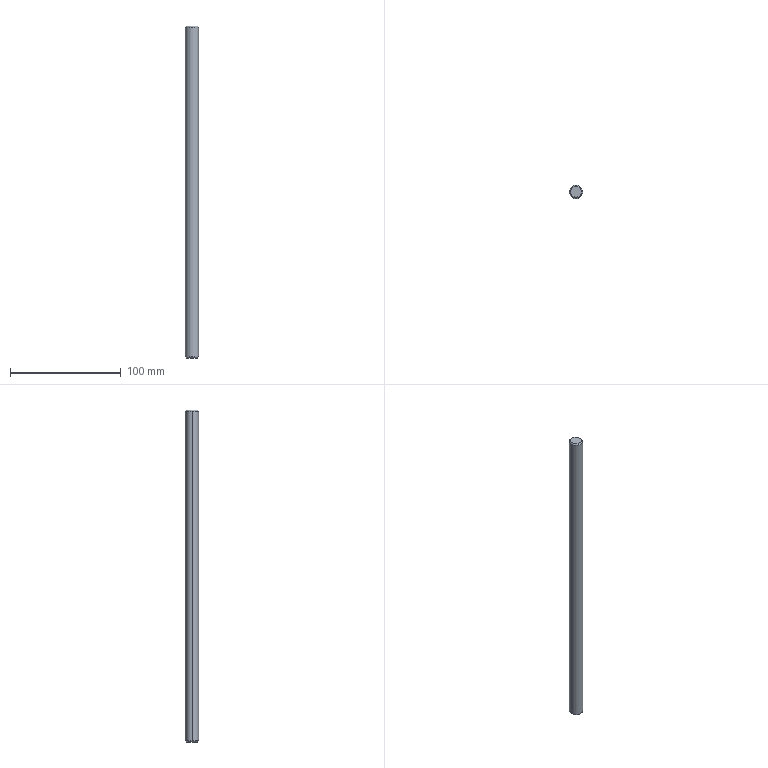Part | STEP file | X77b-01009 | 1 solid | 8 faces | box 12 x 12 x 300 mm | volume 33894 mm3 | cone 4 | cylinder 2 | plane 2 | commonest cylinder face diameters 12 x2
STEP:
#1=CARTESIAN_POINT('',(5.,2660.092,300.));
#2=VERTEX_POINT('',#1);
#3=CARTESIAN_POINT('',(-5.,2660.092,300.));
#4=VERTEX_POINT('',#3);
#5=CARTESIAN_POINT('',(0.000000001,2660.092,300.));
#6=DIRECTION('',(0.,0.,1.));
#7=DIRECTION('',(1.,0.,0.));
#8=AXIS2_PLACEMENT_3D('',#5,#6,#7);
#9=CIRCLE('',#8,5.);
#10=EDGE_CURVE('',#2,#4,#9,.T.);
#11=ORIENTED_EDGE('',*,*,#10,.F.);
#12=CARTESIAN_POINT('',(6.,2660.092,299.));
#13=VERTEX_POINT('',#12);
#14=CARTESIAN_POINT('',(5.,2660.092,300.));
#15=DIRECTION('',(0.7071,0.,-0.7071));
#16=VECTOR('',#15,1000.);
#17=LINE('',#14,#16);
#18=EDGE_CURVE('',#2,#13,#17,.T.);
#19=ORIENTED_EDGE('',*,*,#18,.T.);
#20=CARTESIAN_POINT('',(-6.,2660.092,299.));
#21=VERTEX_POINT('',#20);
#22=CARTESIAN_POINT('',(0.000000001,2660.092,299.));
#23=DIRECTION('',(0.,0.,-1.));
#24=DIRECTION('',(1.,0.,0.));
#25=AXIS2_PLACEMENT_3D('',#22,#23,#24);
#26=CIRCLE('',#25,6.);
#27=EDGE_CURVE('',#21,#13,#26,.T.);
#28=ORIENTED_EDGE('',*,*,#27,.F.);
#29=CARTESIAN_POINT('',(-5.,2660.092,300.));
#30=DIRECTION('',(-0.7071,0.,-0.7071));
#31=VECTOR('',#30,1000.);
#32=LINE('',#29,#31);
#33=EDGE_CURVE('',#4,#21,#32,.T.);
#34=ORIENTED_EDGE('',*,*,#33,.F.);
#35=EDGE_LOOP('',(#11,#19,#28,#34));
#36=FACE_OUTER_BOUND('',#35,.T.);
#37=CARTESIAN_POINT('',(0.000000001,2660.092,300.));
#38=DIRECTION('',(0.,0.,-1.));
#39=DIRECTION('',(-1.,0.,0.));
#40=AXIS2_PLACEMENT_3D('',#37,#38,#39);
#41=CONICAL_SURFACE('',#40,5.,0.7854);
#42=ADVANCED_FACE('',(#36),#41,.T.);
#43=CARTESIAN_POINT('',(-5.,2660.092,0.));
#44=VERTEX_POINT('',#43);
#45=CARTESIAN_POINT('',(5.,2660.092,0.));
#46=VERTEX_POINT('',#45);
#47=CARTESIAN_POINT('',(0.000000001,2660.092,0.));
#48=DIRECTION('',(0.,0.,-1.));
#49=DIRECTION('',(1.,0.,0.));
#50=AXIS2_PLACEMENT_3D('',#47,#48,#49);
#51=CIRCLE('',#50,5.);
#52=EDGE_CURVE('',#44,#46,#51,.T.);
#53=ORIENTED_EDGE('',*,*,#52,.F.);
#54=CARTESIAN_POINT('',(-6.,2660.092,1.));
#55=VERTEX_POINT('',#54);
#56=CARTESIAN_POINT('',(-6.,2660.092,1.));
#57=DIRECTION('',(-0.7071,0.,0.7071));
#58=VECTOR('',#57,1000.);
#59=LINE('',#56,#58);
#60=EDGE_CURVE('',#44,#55,#59,.T.);
#61=ORIENTED_EDGE('',*,*,#60,.T.);
#62=CARTESIAN_POINT('',(6.,2660.092,1.));
#63=VERTEX_POINT('',#62);
#64=CARTESIAN_POINT('',(0.000000001,2660.092,1.));
#65=DIRECTION('',(0.,0.,1.));
#66=DIRECTION('',(1.,0.,0.));
#67=AXIS2_PLACEMENT_3D('',#64,#65,#66);
#68=CIRCLE('',#67,6.);
#69=EDGE_CURVE('',#63,#55,#68,.T.);
#70=ORIENTED_EDGE('',*,*,#69,.F.);
#71=CARTESIAN_POINT('',(6.,2660.092,1.));
#72=DIRECTION('',(0.7071,0.,0.7071));
#73=VECTOR('',#72,1000.);
#74=LINE('',#71,#73);
#75=EDGE_CURVE('',#46,#63,#74,.T.);
#76=ORIENTED_EDGE('',*,*,#75,.F.);
#77=EDGE_LOOP('',(#53,#61,#70,#76));
#78=FACE_OUTER_BOUND('',#77,.T.);
#79=CARTESIAN_POINT('',(0.000000001,2660.092,1.));
#80=DIRECTION('',(0.,0.,1.));
#81=DIRECTION('',(1.,0.,0.));
#82=AXIS2_PLACEMENT_3D('',#79,#80,#81);
#83=CONICAL_SURFACE('',#82,6.,0.7854);
#84=ADVANCED_FACE('',(#78),#83,.T.);
#85=ORIENTED_EDGE('',*,*,#27,.T.);
#86=CARTESIAN_POINT('',(6.,2660.092,300.));
#87=DIRECTION('',(0.,0.,-1.));
#88=VECTOR('',#87,1000.);
#89=LINE('',#86,#88);
#90=EDGE_CURVE('',#13,#63,#89,.T.);
#91=ORIENTED_EDGE('',*,*,#90,.T.);
#92=ORIENTED_EDGE('',*,*,#69,.T.);
#93=CARTESIAN_POINT('',(-6.,2660.092,300.));
#94=DIRECTION('',(0.,0.,-1.));
#95=VECTOR('',#94,1000.);
#96=LINE('',#93,#95);
#97=EDGE_CURVE('',#21,#55,#96,.T.);
#98=ORIENTED_EDGE('',*,*,#97,.F.);
#99=EDGE_LOOP('',(#85,#91,#92,#98));
#100=FACE_OUTER_BOUND('',#99,.T.);
#101=CARTESIAN_POINT('',(0.000000001,2660.092,300.));
#102=DIRECTION('',(0.,0.,-1.));
#103=DIRECTION('',(-1.,0.,0.));
#104=AXIS2_PLACEMENT_3D('',#101,#102,#103);
#105=CYLINDRICAL_SURFACE('',#104,6.);
#106=ADVANCED_FACE('',(#100),#105,.T.);
#107=ORIENTED_EDGE('',*,*,#90,.F.);
#108=CARTESIAN_POINT('',(0.000000001,2660.092,299.));
#109=DIRECTION('',(0.,0.,-1.));
#110=DIRECTION('',(1.,0.,0.));
#111=AXIS2_PLACEMENT_3D('',#108,#109,#110);
#112=CIRCLE('',#111,6.);
#113=EDGE_CURVE('',#13,#21,#112,.T.);
#114=ORIENTED_EDGE('',*,*,#113,.T.);
#115=ORIENTED_EDGE('',*,*,#97,.T.);
#116=CARTESIAN_POINT('',(0.000000001,2660.092,1.));
#117=DIRECTION('',(0.,0.,1.));
#118=DIRECTION('',(1.,0.,0.));
#119=AXIS2_PLACEMENT_3D('',#116,#117,#118);
#120=CIRCLE('',#119,6.);
#121=EDGE_CURVE('',#55,#63,#120,.T.);
#122=ORIENTED_EDGE('',*,*,#121,.T.);
#123=EDGE_LOOP('',(#107,#114,#115,#122));
#124=FACE_OUTER_BOUND('',#123,.T.);
#125=CARTESIAN_POINT('',(0.000000001,2660.092,300.));
#126=DIRECTION('',(0.,0.,-1.));
#127=DIRECTION('',(-1.,0.,0.));
#128=AXIS2_PLACEMENT_3D('',#125,#126,#127);
#129=CYLINDRICAL_SURFACE('',#128,6.);
#130=ADVANCED_FACE('',(#124),#129,.T.);
#131=CARTESIAN_POINT('',(0.000000001,2660.092,300.));
#132=DIRECTION('',(0.,0.,1.));
#133=DIRECTION('',(1.,0.,0.));
#134=AXIS2_PLACEMENT_3D('',#131,#132,#133);
#135=CIRCLE('',#134,5.);
#136=EDGE_CURVE('',#4,#2,#135,.T.);
#137=ORIENTED_EDGE('',*,*,#136,.T.);
#138=ORIENTED_EDGE('',*,*,#10,.T.);
#139=EDGE_LOOP('',(#137,#138));
#140=FACE_OUTER_BOUND('',#139,.T.);
#141=CARTESIAN_POINT('',(0.000000001,2660.092,300.));
#142=DIRECTION('',(0.,0.,1.));
#143=DIRECTION('',(1.,0.,0.));
#144=AXIS2_PLACEMENT_3D('',#141,#142,#143);
#145=PLANE('',#144);
#146=ADVANCED_FACE('',(#140),#145,.T.);
#147=CARTESIAN_POINT('',(0.000000001,2660.092,0.));
#148=DIRECTION('',(0.,0.,-1.));
#149=DIRECTION('',(1.,0.,0.));
#150=AXIS2_PLACEMENT_3D('',#147,#148,#149);
#151=CIRCLE('',#150,5.);
#152=EDGE_CURVE('',#46,#44,#151,.T.);
#153=ORIENTED_EDGE('',*,*,#152,.T.);
#154=ORIENTED_EDGE('',*,*,#52,.T.);
#155=EDGE_LOOP('',(#153,#154));
#156=FACE_OUTER_BOUND('',#155,.T.);
#157=CARTESIAN_POINT('',(0.000000001,2660.092,0.));
#158=DIRECTION('',(0.,0.,1.));
#159=DIRECTION('',(1.,0.,0.));
#160=AXIS2_PLACEMENT_3D('',#157,#158,#159);
#161=PLANE('',#160);
#162=ADVANCED_FACE('',(#156),#161,.F.);
#163=ORIENTED_EDGE('',*,*,#60,.F.);
#164=ORIENTED_EDGE('',*,*,#152,.F.);
#165=ORIENTED_EDGE('',*,*,#75,.T.);
#166=ORIENTED_EDGE('',*,*,#121,.F.);
#167=EDGE_LOOP('',(#163,#164,#165,#166));
#168=FACE_OUTER_BOUND('',#167,.T.);
#169=CARTESIAN_POINT('',(0.000000001,2660.092,1.));
#170=DIRECTION('',(0.,0.,1.));
#171=DIRECTION('',(1.,0.,0.));
#172=AXIS2_PLACEMENT_3D('',#169,#170,#171);
#173=CONICAL_SURFACE('',#172,6.,0.7854);
#174=ADVANCED_FACE('',(#168),#173,.T.);
#175=ORIENTED_EDGE('',*,*,#18,.F.);
#176=ORIENTED_EDGE('',*,*,#136,.F.);
#177=ORIENTED_EDGE('',*,*,#33,.T.);
#178=ORIENTED_EDGE('',*,*,#113,.F.);
#179=EDGE_LOOP('',(#175,#176,#177,#178));
#180=FACE_OUTER_BOUND('',#179,.T.);
#181=CARTESIAN_POINT('',(0.000000001,2660.092,300.));
#182=DIRECTION('',(0.,0.,-1.));
#183=DIRECTION('',(-1.,0.,0.));
#184=AXIS2_PLACEMENT_3D('',#181,#182,#183);
#185=CONICAL_SURFACE('',#184,5.,0.7854);
#186=ADVANCED_FACE('',(#180),#185,.T.);
#187=CLOSED_SHELL('',(#42,#84,#106,#130,#146,#162,#174,#186));
#188=MANIFOLD_SOLID_BREP('',#187);
#189=CARTESIAN_POINT('',(0.,0.,0.));
#190=DIRECTION('',(0.,0.,1.));
#191=DIRECTION('',(1.,0.,0.));
#192=AXIS2_PLACEMENT_3D('',#189,#190,#191);
#193=(LENGTH_UNIT()NAMED_UNIT(*)SI_UNIT(.MILLI.,.METRE.));
#194=UNCERTAINTY_MEASURE_WITH_UNIT(LENGTH_MEASURE(0.00001),#193,'','');
#195=(NAMED_UNIT(*)PLANE_ANGLE_UNIT()SI_UNIT($,.RADIAN.));
#196=(NAMED_UNIT(*)SI_UNIT($,.STERADIAN.)SOLID_ANGLE_UNIT());
#197=(GEOMETRIC_REPRESENTATION_CONTEXT(3)GLOBAL_UNCERTAINTY_ASSIGNED_CONTEXT((#194))GLOBAL_UNIT_ASSIGNED_CONTEXT((#193,#195,#196))REPRESENTATION_CONTEXT('',''));
#198=ADVANCED_BREP_SHAPE_REPRESENTATION('',(#188,#192),#197);